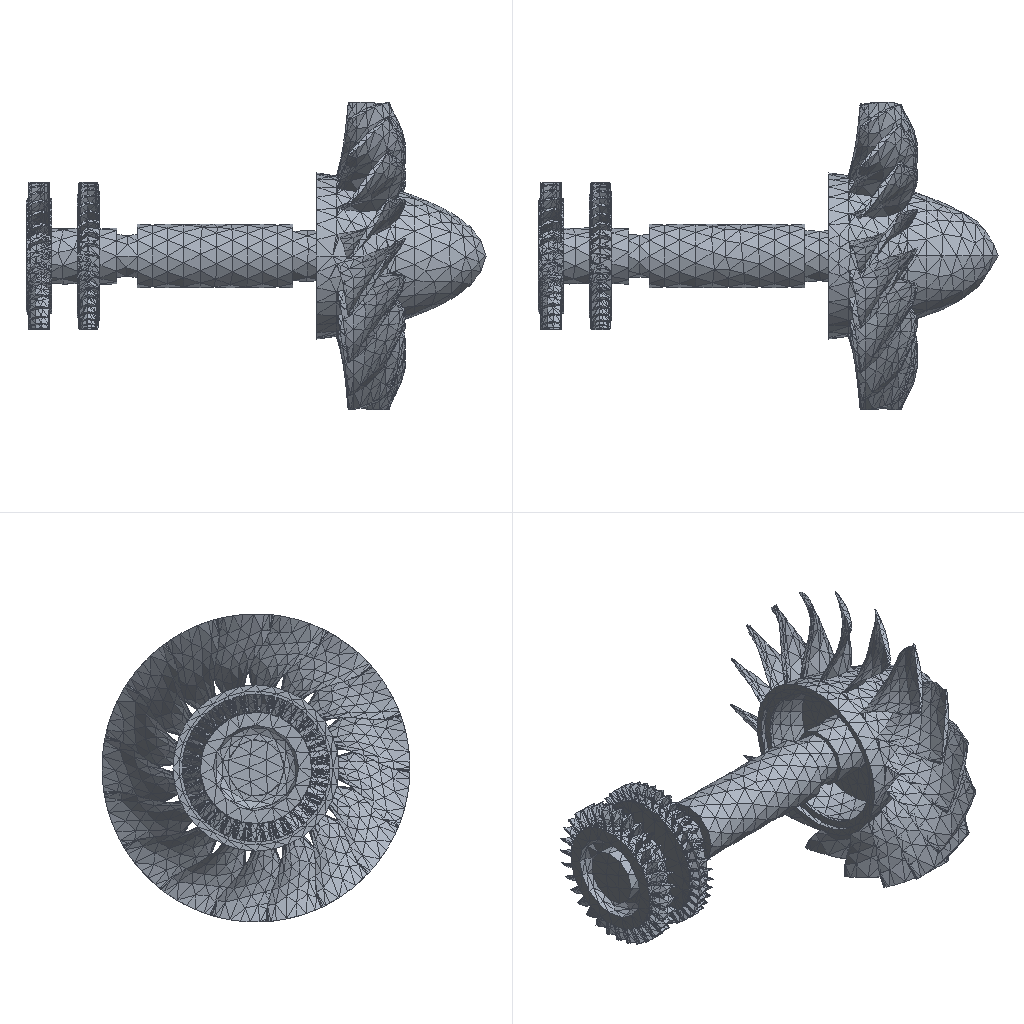Simulation study | ansys workbench
Ansys APDL input file, long lists of numbers shortened:
/batch
/config,noeldb,1     ! force off writing results to database
*get,_wallstrt,active,,time,wall
! ANSYS input file written by Workbench version 2021 R2
! File used for geometry attach:
/title,wbnew--__ (B5)
! ****** Begin Custom Load Command Snippet ******
/COM, ACT Extensions:
/COM,     LSDYNA, 2021.1
/COM,
! ****** End   Custom Load Command Snippet ******
*DIM,_wb_ProjectScratch_dir,string,248
_wb_ProjectScratch_dir(1) = ''
*DIM,_wb_SolverFiles_dir,string,248
_wb_SolverFiles_dir(1) = ''
*DIM,_wb_userfiles_dir,string,248
_wb_userfiles_dir(1) = ''
/com,--- Data in consistent NMM units. See Solving Units in the help system for more information.
/units,MPA
/nopr
/wb,file,start              !  signify a WB generated input file
/prep7
! Turn off shape checking because checks already performed inside WB mesher.
! See help system for more information.
SHPP,OFF,,NOWARN
/nolist
etcon,set             ! allow ANSYS to choose best KEYOP's for 180x elements, resets any applicable keyopt to MAPDL defaults
/com,*********** Nodes for the whole assembly ***********
nblock,3,,62398
(1i9,3e20.9e3)
        1    -4.700000000E+01    -1.870000000E+01     4.580103396E-15
! (56725 more lines like these left out)
-1
/com,*********** Nodes for all Remote Points ***********
nblock,3
(1i9,3e20.9e3)
    56727     0.000000000E+00     0.000000000E+00     0.000000000E+00
! (7 more lines like these left out)
-1
/wb,elem,start            !  set before creation of elements
/com,*********** Elements for Body 1 "Component1\0600" ***********
et,1,187
eblock,19,solid,,8713
(19i9)
        1        1        1        1        0        0        0        0       10        0    10703    21485    21806    23978    21486    27955    29790    27961    27951
! (17425 more lines like these left out)
-1
/com,*********** Elements for Body 2 "Component2\710500" ***********
et,2,187
eblock,19,solid,,1903
(19i9)
        2        2        2        2        0        0        0        0       10        0        1       53      516      103      466      898     1186      892      897
! (3805 more lines like these left out)
-1
/com,*********** Elements for Body 3 "Component3\2R710N21" ***********
et,3,187
eblock,19,solid,,8799
(19i9)
        3        3        3        3        0        0        0        0       10        0     1904     3782     6313     4252     6312    10973    14295    10966    10972
! (17597 more lines like these left out)
-1
/com,*********** Elements for Body 4 "Component4\1R710N411" ***********
et,4,187
eblock,19,solid,,8012
(19i9)
        4        4        4        4        0        0        0        0       10        0    19416    39967    42150    42172    42169    50334    56718    50336    50335
! (16023 more lines like these left out)
-1
/wb,elem,end               !  done creating elements
/com,*********** Send User Defined Coordinate System(s) ***********
csys,0
toffst,273.15,  ! Temperature offset from absolute zero
/com,*********** Set Reference Temperature ***********
tref,22.
/wb,mat,start              !  starting to send materials
/com,*********** Send Materials ***********
Temperature = 'TEMP' ! Temperature
MP,DENS,1,7.85e-09,	! tonne mm^-3
MP,ALPX,1,1.2e-05,	! C^-1
MP,C,1,434000000,	! mm^2 s^-2 C^-1
MP,KXX,1,60.5,	! tonne mm s^-3 C^-1
MP,RSVX,1,0.00017,	! ohm mm
MP,EX,1,200000,	! tonne s^-2 mm^-1
MP,NUXY,1,0.3,
MP,MURX,1,10000,
Temperature = 'TEMP' ! Temperature
MP,DENS,2,7.85e-09,	! tonne mm^-3
MP,ALPX,2,1.2e-05,	! C^-1
MP,C,2,434000000,	! mm^2 s^-2 C^-1
MP,KXX,2,60.5,	! tonne mm s^-3 C^-1
MP,RSVX,2,0.00017,	! ohm mm
MP,EX,2,200000,	! tonne s^-2 mm^-1
MP,NUXY,2,0.3,
MP,MURX,2,10000,
Temperature = 'TEMP' ! Temperature
MP,DENS,3,7.85e-09,	! tonne mm^-3
MP,ALPX,3,1.2e-05,	! C^-1
MP,C,3,434000000,	! mm^2 s^-2 C^-1
MP,KXX,3,60.5,	! tonne mm s^-3 C^-1
MP,RSVX,3,0.00017,	! ohm mm
MP,EX,3,200000,	! tonne s^-2 mm^-1
MP,NUXY,3,0.3,
MP,MURX,3,10000,
Temperature = 'TEMP' ! Temperature
MP,DENS,4,7.85e-09,	! tonne mm^-3
MP,ALPX,4,1.2e-05,	! C^-1
MP,C,4,434000000,	! mm^2 s^-2 C^-1
MP,KXX,4,60.5,	! tonne mm s^-3 C^-1
MP,RSVX,4,0.00017,	! ohm mm
MP,EX,4,200000,	! tonne s^-2 mm^-1
MP,NUXY,4,0.3,
MP,MURX,4,10000,
/wb,mat,end                !  done sending materials
!************************* Model Summary ********************
!Component1\0600,	结构钢,	matid,	1
!Component2\710500,	结构钢,	matid,	2
!Component3\2R710N21,	结构钢,	matid,	3
!Component4\1R710N411,	结构钢,	matid,	4
!************************* End Model Summary ********************
! get the diagonal of the bounding box. Needed later for other things
*get,_xmin,node,,mnloc,x
*get,_ymin,node,,mnloc,y
*get,_zmin,node,,mnloc,z
*get,_xmax,node,,mxloc,x
*get,_ymax,node,,mxloc,y
*get,_zmax,node,,mxloc,z
_ASMDIAG=(_xmax-_xmin)*(_xmax-_xmin)+(_ymax-_ymin)*(_ymax-_ymin)+(_zmax-_zmin)*(_zmax-_zmin)
_ASMDIAG=SQRT(_ASMDIAG)
/wb,contact,start          !  starting to send contact
/com,*********** Create Contact "接触区域" ***********
/com,            Real Constant Set For Above Contact Is 6 & 5
*set,tid,6
*set,cid,5
r,tid
r,cid
et,tid,170
et,cid,174
eblock,10,,,46
(15i9)
    45624        6        6        6        0    21704    21705    23800    23800    29061    29069    23800    29062
! (45 more lines like these left out)
-1
eblock,10,,,46
(15i9)
    45670        5        5        5        0    21704    21705    23800    23800    29061    29069    23800    29062
! (45 more lines like these left out)
-1
eblock,10,,,66
(15i9)
    45716        5        6        5        0       92       91      123      123     1129     1130      123     1136
! (65 more lines like these left out)
-1
eblock,10,,,66
(15i9)
    45782        6        5        6        0       92       91      123      123     1129     1130      123     1136
! (65 more lines like these left out)
-1
keyo,cid,8,2               ! auto create asymmetric contact (from Program Controlled setting)
keyo,cid,10,0              ! adjust contact stiffness each NR iteration (from Program Controlled setting)
keyo,cid,12,5              ! bonded always
keyo,cid,18,1              ! small sliding turned on by application
keyo,cid,2,0               ! augmented Lagrange (from Program Controlled setting)
keyo,cid,4,0               ! on Gauss point (from Program Controlled setting)
keyo,cid,9,1               ! ignore initial gaps/penetration
keyo,cid,7,0               ! No Prediction
rmod,tid,3,10.      ! FKN
rmod,tid,5,0.       ! ICONT
rmod,tid,6,0.       ! PINB
rmod,tid,10,0.      ! CNOF
rmod,tid,12,0.      ! FKT
rmod,tid,36,33      ! WB DSID
rmod,cid,3,10.      ! FKN
rmod,cid,5,0.       ! ICONT
rmod,cid,6,0.       ! PINB
rmod,cid,10,0.      ! CNOF
rmod,cid,12,0.      ! FKT
rmod,cid,36,33      ! WB DSID
/com,*********** Create Contact "接触区域 2" ***********
/com,            Real Constant Set For Above Contact Is 8 & 7
*set,tid,8
*set,cid,7
r,tid
r,cid
et,tid,170
et,cid,174
eblock,10,,,44
(15i9)
    45848        8        8        8        0       71       61      165      165      965      967      165     1038
! (43 more lines like these left out)
-1
eblock,10,,,44
(15i9)
    45892        7        7        7        0       71       61      165      165      965      967      165     1038
! (43 more lines like these left out)
-1
eblock,10,,,22
(15i9)
    45936        7        8        7        0     3558     3568     3579     3579     8685     8739     3579     8688
! (21 more lines like these left out)
-1
eblock,10,,,22
(15i9)
    45958        8        7        8        0     3558     3568     3579     3579     8685     8739     3579     8688
! (21 more lines like these left out)
-1
keyo,cid,8,2               ! auto create asymmetric contact (from Program Controlled setting)
keyo,cid,10,0              ! adjust contact stiffness each NR iteration (from Program Controlled setting)
keyo,cid,12,5              ! bonded always
keyo,cid,18,1              ! small sliding turned on by application
keyo,cid,2,0               ! augmented Lagrange (from Program Controlled setting)
keyo,cid,4,0               ! on Gauss point (from Program Controlled setting)
keyo,cid,9,1               ! ignore initial gaps/penetration
keyo,cid,7,0               ! No Prediction
rmod,tid,3,10.      ! FKN
rmod,tid,5,0.       ! ICONT
rmod,tid,6,0.       ! PINB
rmod,tid,10,0.      ! CNOF
rmod,tid,12,0.      ! FKT
rmod,tid,36,36      ! WB DSID
rmod,cid,3,10.      ! FKN
rmod,cid,5,0.       ! ICONT
rmod,cid,6,0.       ! PINB
rmod,cid,10,0.      ! CNOF
rmod,cid,12,0.      ! FKT
rmod,cid,36,36      ! WB DSID
/com,*********** Create Contact "接触区域 3" ***********
/com,            Real Constant Set For Above Contact Is 10 & 9
*set,tid,10
*set,cid,9
r,tid
r,cid
et,tid,170
et,cid,174
eblock,10,,,66
(15i9)
    45980       10       10       10        0       72       82      166      166     1042     1082      166     1043
! (65 more lines like these left out)
-1
eblock,10,,,66
(15i9)
    46046        9        9        9        0       72       82      166      166     1042     1082      166     1043
! (65 more lines like these left out)
-1
eblock,10,,,36
(15i9)
    46112        9       10        9        0    39377    39387    41892    41892    47458    47514    41892    47460
! (35 more lines like these left out)
-1
eblock,10,,,36
(15i9)
    46148       10        9       10        0    39377    39387    41892    41892    47458    47514    41892    47460
! (35 more lines like these left out)
-1
keyo,cid,8,2               ! auto create asymmetric contact (from Program Controlled setting)
keyo,cid,10,0              ! adjust contact stiffness each NR iteration (from Program Controlled setting)
keyo,cid,12,5              ! bonded always
keyo,cid,18,1              ! small sliding turned on by application
keyo,cid,2,0               ! augmented Lagrange (from Program Controlled setting)
keyo,cid,4,0               ! on Gauss point (from Program Controlled setting)
keyo,cid,9,1               ! ignore initial gaps/penetration
keyo,cid,7,0               ! No Prediction
rmod,tid,3,10.      ! FKN
rmod,tid,5,0.       ! ICONT
rmod,tid,6,0.       ! PINB
rmod,tid,10,0.      ! CNOF
rmod,tid,12,0.      ! FKT
rmod,tid,36,39      ! WB DSID
rmod,cid,3,10.      ! FKN
rmod,cid,5,0.       ! ICONT
rmod,cid,6,0.       ! PINB
rmod,cid,10,0.      ! CNOF
rmod,cid,12,0.      ! FKT
rmod,cid,36,39      ! WB DSID
nsel,all
esel,all
/wb,contact,end            !  done creating contacts
/golist
/wb,load,start             !  starting to send loads
/com,*********** Create Remote Point "内部远程点 2" ***********
! -------- Remote Point Used by "接地 至 Component2\710500" --------
*set,tid,12
*set,cid,11
et,cid,174
et,tid,170
keyo,tid,2,1               ! Don't fix the pilot node
keyo,tid,4,111111
keyo,cid,12,5              ! Bonded Contact
keyo,cid,4,2               ! Rigid CERIG style load
keyo,cid,2,2               ! MPC style contact
eblock,10,,,40
(15i9)
    46184       11       11       11        0       59       60      211      211      947      959      211      951
! (39 more lines like these left out)
-1
*set,_npilot,56728
_npilot49=_npilot
type,tid
mat ,cid
real,cid
tshape,pilo
en,46224,_npilot
tshape
/com,*********** Create Remote Point "内部远程点 4" ***********
! -------- Remote Point Used by "接地 至 Component2\710500" --------
*set,tid,14
*set,cid,13
et,cid,174
et,tid,170
keyo,tid,2,1               ! Don't fix the pilot node
keyo,tid,4,111111
keyo,cid,12,5              ! Bonded Contact
keyo,cid,4,2               ! Rigid CERIG style load
keyo,cid,2,2               ! MPC style contact
eblock,10,,,30
(15i9)
    46225       13       13       13        0       30       31      220      220      699      715      220      704
! (29 more lines like these left out)
-1
*set,_npilot,56731
_npilot53=_npilot
type,tid
mat ,cid
real,cid
tshape,pilo
en,46255,_npilot
tshape
/com,*********** Create Remote Point "内部远程点 6" ***********
! -------- Remote Point Used by "远程位移" --------
*set,tid,16
*set,cid,15
et,cid,174
et,tid,170
keyo,tid,2,1               ! Don't fix the pilot node
keyo,tid,4,111111
keyo,cid,12,5              ! Bonded Contact
keyo,cid,4,2               ! Rigid CERIG style load
keyo,cid,2,2               ! MPC style contact
eblock,10,,,19
(15i9)
    46256       15       15       15        0       66      339       67       67     1001     1010       67      995
! (18 more lines like these left out)
-1
*set,_npilot,56733
_npilot63=_npilot
type,tid
mat ,cid
real,cid
tshape,pilo
en,46275,_npilot
tshape
/com,*********** Create Remote Point "内部远程点 7" ***********
! -------- Remote Point Used by "远程位移 2" --------
*set,tid,18
*set,cid,17
et,cid,174
et,tid,170
keyo,tid,2,1               ! Don't fix the pilot node
keyo,tid,4,111111
keyo,cid,12,5              ! Bonded Contact
keyo,cid,4,2               ! Rigid CERIG style load
keyo,cid,2,2               ! MPC style contact
eblock,10,,,19
(15i9)
    46276       17       17       17        0      343      344      345      345     2529     2537      345     2530
! (18 more lines like these left out)
-1
*set,_npilot,56734
_npilot66=_npilot
type,tid
mat ,cid
real,cid
tshape,pilo
en,46295,_npilot
tshape
/com,*********** Create Bearing Connection "接地 至 Component2\710500" ***********
!
! Setup Bearing Connection For Reference Set which is Grounded
d,56729,all
/com,            Real Constant Set For Above Bearing Connection Is 19
*set,_sid,19
et,_sid,214            ! Combi214, Bearing-Damper Element
keyo,_sid,2,1     ! YZ Plane
keyo,_sid,3,0     ! Symmetric [K] and [C]
r,_sid,10000.,10000.,0.,0.,0.,0.
rmore,0.,0.
mat,_sid
real,_sid
type,_sid
en,45616,56729,56728
/com,*********** Create Bearing Connection "接地 至 Component2\710500" ***********
!
! Setup Bearing Connection For Reference Set which is Grounded
d,56732,all
/com,            Real Constant Set For Above Bearing Connection Is 20
*set,_sid,20
et,_sid,214            ! Combi214, Bearing-Damper Element
keyo,_sid,2,1     ! YZ Plane
keyo,_sid,3,0     ! Symmetric [K] and [C]
r,_sid,10000.,10000.,0.,0.,0.,0.
rmore,0.,0.
mat,_sid
real,_sid
type,_sid
en,45617,56732,56731
/com,*********** Construct Remote Displacement ***********
*DIM,_loadvari62ux,TABLE,1,1,1,TIME
! Time values
*TAXIS,_loadvari62ux(1),1,1.
! Load values
_loadvari62ux(1,1,1) = 0.
/com,*********** Construct Remote Displacement ***********
*DIM,_loadvari65ux,TABLE,1,1,1,TIME
! Time values
*TAXIS,_loadvari65ux(1),1,1.
! Load values
_loadvari65ux(1,1,1) = 0.
d,56733,ux,%_loadvari62ux%
d,56734,ux,%_loadvari65ux%
/COM,*** Create a component for all remote displacements ***
CMBLOCK,REMOTEDISPALL,NODE,        2
(8i10)
     56733     56734
/gst,on,on
fini
*get,_numnode,node,0,count
*get,_numelem,elem,0,count
*get, _MAXELEMNUM, elem, 0, NUM, MAX
*get, _MAXNODENUM, node, 0, NUM, MAX
*get, _MAXELEMTYPE, etyp, 0, NUM, MAX
*get, _MAXREALCONST, real, 0, NUM, MAX
/go
/wb,load,end               !  done creating loads
/com,--- Number of total nodes = %_numnode%
/com,--- Number of contact elements = 668
/com,--- Number of spring elements = 0
/com,--- Number of bearing elements = 0
/com,--- Number of solid elements = 27427
/com,--- Number of condensed parts = 0
/com,--- Number of total elements = %_numelem%
*get,_wallbsol,active,,time,wall
/solu
antype,2                   ! modal analysis
_thickRatio=0.5     ! Ratio of thick parts in the model
modopt,lanb,4
outres,erase
outres,all,none
outres,nsol,all
outres,etmp,all
/nopr
esel,s,type,,19
esel,a,type,,20
cm,_elmisc,elem
esel,all
/gopr
outres,misc,all,_elmisc
mxpand,,,,yes,,no             ! expand requested element results, but not write them to file.mode
dmpopt,esav,no
dmpopt,emat,no
dmpopt,full,no
! *********** WB SOLVE COMMAND ***********
! check interactive state
*get,ANSINTER_,active,,int
*if,ANSINTER_,ne,0,then
/eof
*endif
solve
/com *************** Write FE CONNECTORS *********
CEWRITE,file,ce,,INTE
*get,_nmodalsolproc,active,0,numcpu
fini
/nopr
*get,_numnode,node,0,count
*get,_numelem,elem,0,count
*get, _MAXELEMNUM, elem, 0, NUM, MAX
*get, _MAXNODENUM, node, 0, NUM, MAX,,,INTERNAL
*get, _MAXELEMTYPE, etyp, 0, NUM, MAX
*get, _MAXREALCONST, real, 0, NUM, MAX
/gopr
*get,_wallasol,active,,time,wall
/post1
/nopr
*dim,_direction,CHAR,6,1
_direction(1) = 'X'
_direction(2) = 'Y'
_direction(3) = 'Z'
_direction(4) = 'ROTX'
_direction(5) = 'ROTY'
_direction(6) = 'ROTZ'
*get,_lastLS,active,0,set,LSTP
*get,_beginset,active,0,set,nset,first,_lastLS
*get,_endset,active,0,set,nset,last,_lastLS
_nummodes = 0
*if,_endset,gt,0,then
_nummodes = _endset - _beginset + 1
*endif
*do,i_mode,1,_nummodes
   *do,j_component,1,6
			*get,PFACT_%i_mode%_%j_component%,MODE,%i_mode%,PFACT,,DIREC,_direction(%j_component%)
   *enddo
*enddo
*dim,_tmdirection,CHAR,6,1
_tmdirection(1) = 'X'
_tmdirection(2) = 'Y'
_tmdirection(3) = 'Z'
_tmdirection(4) = 'X'
_tmdirection(5) = 'Y'
_tmdirection(6) = 'Z'
*do,j_component,1,6
    *if,j_component,gt,3,then
        *get,TOTALMASS_%j_component%,ELEM,0,IOR,_tmdirection(%j_component%)
    *else
        *get,TOTALMASS_%j_component%,ELEM,0,MTOT,_tmdirection(%j_component%)
    *endif
*enddo
/gopr
xmlo,ENCODING,ISO-8859-1
xmlo,parm
/xml,parm,xml
fini
/gopr
*get,_walldone,active,,time,wall
_preptime=(_wallbsol-_wallstrt)*3600
_solvtime=(_wallasol-_wallbsol)*3600
_posttime=(_walldone-_wallasol)*3600
_totaltim=(_walldone-_wallstrt)*3600
*get,_dlbratio,active,0,solu,dlbr
*get,_combtime,active,0,solu,comb
*get,_ssmode,active,0,solu,ssmm
*get,_ndofs,active,0,solu,ndof
/com,--- Total number of nodes = %_numnode%
/com,--- Total number of elements = %_numelem%
/com,--- Element load balance ratio = %_dlbratio%
/com,--- Time to combine distributed files = %_combtime%
/com,--- Sparse memory mode = %_ssmode%
/com,--- Number of DOF = %_ndofs%
/wb,file,end               ! done with WB generated input